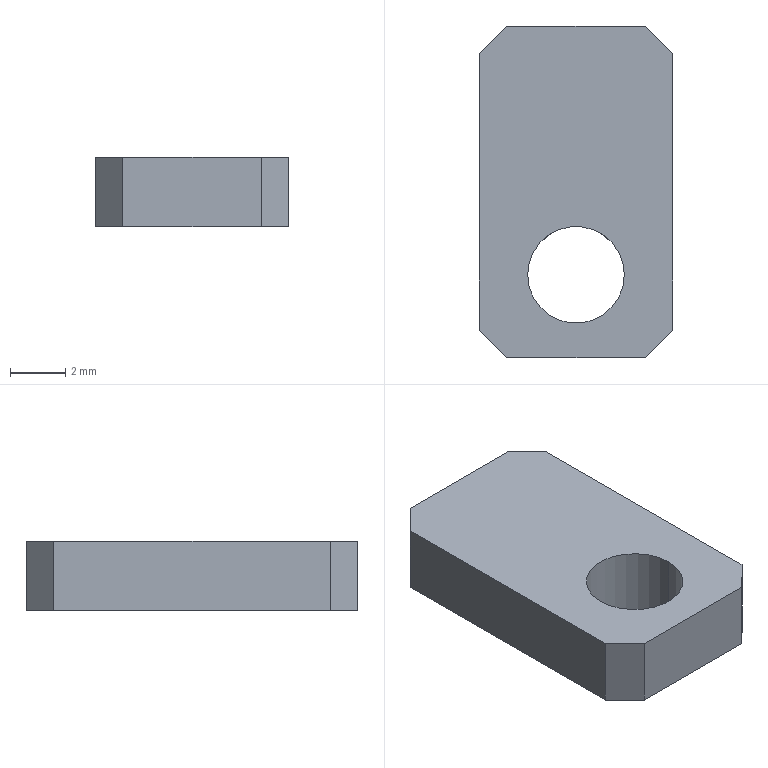Part | SolidWorks | features Chamfer 1, Extrusion 1, HoleWzd 1 | 1 solid | 12 faces | box 7 x 12 x 2.5 mm | volume 180.947 mm3 | plane 10 | cylinder 2 | commonest cylinder face diameters 3.5 x2
STEP:
#1=CARTESIAN_POINT('',(-1.75,-3.,-1.25));
#2=VERTEX_POINT('',#1);
#3=CARTESIAN_POINT('',(1.75,-3.,-1.25));
#4=VERTEX_POINT('',#3);
#5=CARTESIAN_POINT('',(0.,-3.,-1.25));
#6=DIRECTION('',(0.,0.,1.));
#7=DIRECTION('',(1.,0.,0.));
#8=AXIS2_PLACEMENT_3D('',#5,#6,#7);
#9=CIRCLE('',#8,1.75);
#10=EDGE_CURVE('',#2,#4,#9,.T.);
#11=ORIENTED_EDGE('',*,*,#10,.F.);
#12=CARTESIAN_POINT('',(-1.75,-3.,1.25));
#13=VERTEX_POINT('',#12);
#14=CARTESIAN_POINT('',(-1.75,-3.,1.25));
#15=DIRECTION('',(0.,0.,1.));
#16=VECTOR('',#15,1000.);
#17=LINE('',#14,#16);
#18=EDGE_CURVE('',#2,#13,#17,.T.);
#19=ORIENTED_EDGE('',*,*,#18,.T.);
#20=CARTESIAN_POINT('',(1.75,-3.,1.25));
#21=VERTEX_POINT('',#20);
#22=CARTESIAN_POINT('',(0.,-3.,1.25));
#23=DIRECTION('',(0.,0.,1.));
#24=DIRECTION('',(1.,0.,0.));
#25=AXIS2_PLACEMENT_3D('',#22,#23,#24);
#26=CIRCLE('',#25,1.75);
#27=EDGE_CURVE('',#13,#21,#26,.T.);
#28=ORIENTED_EDGE('',*,*,#27,.T.);
#29=CARTESIAN_POINT('',(1.75,-3.,1.25));
#30=DIRECTION('',(0.,0.,1.));
#31=VECTOR('',#30,1000.);
#32=LINE('',#29,#31);
#33=EDGE_CURVE('',#4,#21,#32,.T.);
#34=ORIENTED_EDGE('',*,*,#33,.F.);
#35=EDGE_LOOP('',(#11,#19,#28,#34));
#36=FACE_OUTER_BOUND('',#35,.T.);
#37=CARTESIAN_POINT('',(0.,-3.,1.25));
#38=DIRECTION('',(0.,0.,1.));
#39=DIRECTION('',(1.,0.,0.));
#40=AXIS2_PLACEMENT_3D('',#37,#38,#39);
#41=CYLINDRICAL_SURFACE('',#40,1.75);
#42=ADVANCED_FACE('',(#36),#41,.F.);
#43=CARTESIAN_POINT('',(3.5,-5.,1.25));
#44=VERTEX_POINT('',#43);
#45=CARTESIAN_POINT('',(3.5,5.,1.25));
#46=VERTEX_POINT('',#45);
#47=CARTESIAN_POINT('',(3.5,6.,1.25));
#48=DIRECTION('',(0.,1.,0.));
#49=VECTOR('',#48,1000.);
#50=LINE('',#47,#49);
#51=EDGE_CURVE('',#44,#46,#50,.T.);
#52=ORIENTED_EDGE('',*,*,#51,.F.);
#53=CARTESIAN_POINT('',(3.5,-5.,-1.25));
#54=VERTEX_POINT('',#53);
#55=CARTESIAN_POINT('',(3.5,-5.,1.25));
#56=DIRECTION('',(0.,0.,-1.));
#57=VECTOR('',#56,1000.);
#58=LINE('',#55,#57);
#59=EDGE_CURVE('',#44,#54,#58,.T.);
#60=ORIENTED_EDGE('',*,*,#59,.T.);
#61=CARTESIAN_POINT('',(3.5,5.,-1.25));
#62=VERTEX_POINT('',#61);
#63=CARTESIAN_POINT('',(3.5,6.,-1.25));
#64=DIRECTION('',(0.,1.,0.));
#65=VECTOR('',#64,1000.);
#66=LINE('',#63,#65);
#67=EDGE_CURVE('',#54,#62,#66,.T.);
#68=ORIENTED_EDGE('',*,*,#67,.T.);
#69=CARTESIAN_POINT('',(3.5,5.,1.25));
#70=DIRECTION('',(0.,0.,1.));
#71=VECTOR('',#70,1000.);
#72=LINE('',#69,#71);
#73=EDGE_CURVE('',#62,#46,#72,.T.);
#74=ORIENTED_EDGE('',*,*,#73,.T.);
#75=EDGE_LOOP('',(#52,#60,#68,#74));
#76=FACE_OUTER_BOUND('',#75,.T.);
#77=CARTESIAN_POINT('',(3.5,6.,1.25));
#78=DIRECTION('',(-1.,0.,0.));
#79=DIRECTION('',(0.,-1.,0.));
#80=AXIS2_PLACEMENT_3D('',#77,#78,#79);
#81=PLANE('',#80);
#82=ADVANCED_FACE('',(#76),#81,.F.);
#83=CARTESIAN_POINT('',(2.5,6.,-1.25));
#84=VERTEX_POINT('',#83);
#85=CARTESIAN_POINT('',(-2.5,6.,-1.25));
#86=VERTEX_POINT('',#85);
#87=CARTESIAN_POINT('',(-3.5,6.,-1.25));
#88=DIRECTION('',(-1.,0.,0.));
#89=VECTOR('',#88,1000.);
#90=LINE('',#87,#89);
#91=EDGE_CURVE('',#84,#86,#90,.T.);
#92=ORIENTED_EDGE('',*,*,#91,.T.);
#93=CARTESIAN_POINT('',(-2.5,6.,1.25));
#94=VERTEX_POINT('',#93);
#95=CARTESIAN_POINT('',(-2.5,6.,1.25));
#96=DIRECTION('',(0.,0.,1.));
#97=VECTOR('',#96,1000.);
#98=LINE('',#95,#97);
#99=EDGE_CURVE('',#86,#94,#98,.T.);
#100=ORIENTED_EDGE('',*,*,#99,.T.);
#101=CARTESIAN_POINT('',(2.5,6.,1.25));
#102=VERTEX_POINT('',#101);
#103=CARTESIAN_POINT('',(-3.5,6.,1.25));
#104=DIRECTION('',(-1.,0.,0.));
#105=VECTOR('',#104,1000.);
#106=LINE('',#103,#105);
#107=EDGE_CURVE('',#102,#94,#106,.T.);
#108=ORIENTED_EDGE('',*,*,#107,.F.);
#109=CARTESIAN_POINT('',(2.5,6.,1.25));
#110=DIRECTION('',(0.,0.,-1.));
#111=VECTOR('',#110,1000.);
#112=LINE('',#109,#111);
#113=EDGE_CURVE('',#102,#84,#112,.T.);
#114=ORIENTED_EDGE('',*,*,#113,.T.);
#115=EDGE_LOOP('',(#92,#100,#108,#114));
#116=FACE_OUTER_BOUND('',#115,.T.);
#117=CARTESIAN_POINT('',(-3.5,6.,1.25));
#118=DIRECTION('',(0.,-1.,0.));
#119=DIRECTION('',(0.,0.,-1.));
#120=AXIS2_PLACEMENT_3D('',#117,#118,#119);
#121=PLANE('',#120);
#122=ADVANCED_FACE('',(#116),#121,.F.);
#123=CARTESIAN_POINT('',(-3.5,5.,-1.25));
#124=VERTEX_POINT('',#123);
#125=CARTESIAN_POINT('',(-3.5,-5.,-1.25));
#126=VERTEX_POINT('',#125);
#127=CARTESIAN_POINT('',(-3.5,6.,-1.25));
#128=DIRECTION('',(0.,-1.,0.));
#129=VECTOR('',#128,1000.);
#130=LINE('',#127,#129);
#131=EDGE_CURVE('',#124,#126,#130,.T.);
#132=ORIENTED_EDGE('',*,*,#131,.T.);
#133=CARTESIAN_POINT('',(-3.5,-5.,1.25));
#134=VERTEX_POINT('',#133);
#135=CARTESIAN_POINT('',(-3.5,-5.,1.25));
#136=DIRECTION('',(0.,0.,1.));
#137=VECTOR('',#136,1000.);
#138=LINE('',#135,#137);
#139=EDGE_CURVE('',#126,#134,#138,.T.);
#140=ORIENTED_EDGE('',*,*,#139,.T.);
#141=CARTESIAN_POINT('',(-3.5,5.,1.25));
#142=VERTEX_POINT('',#141);
#143=CARTESIAN_POINT('',(-3.5,6.,1.25));
#144=DIRECTION('',(0.,-1.,0.));
#145=VECTOR('',#144,1000.);
#146=LINE('',#143,#145);
#147=EDGE_CURVE('',#142,#134,#146,.T.);
#148=ORIENTED_EDGE('',*,*,#147,.F.);
#149=CARTESIAN_POINT('',(-3.5,5.,1.25));
#150=DIRECTION('',(0.,0.,-1.));
#151=VECTOR('',#150,1000.);
#152=LINE('',#149,#151);
#153=EDGE_CURVE('',#142,#124,#152,.T.);
#154=ORIENTED_EDGE('',*,*,#153,.T.);
#155=EDGE_LOOP('',(#132,#140,#148,#154));
#156=FACE_OUTER_BOUND('',#155,.T.);
#157=CARTESIAN_POINT('',(-3.5,6.,1.25));
#158=DIRECTION('',(1.,0.,0.));
#159=DIRECTION('',(0.,1.,0.));
#160=AXIS2_PLACEMENT_3D('',#157,#158,#159);
#161=PLANE('',#160);
#162=ADVANCED_FACE('',(#156),#161,.F.);
#163=CARTESIAN_POINT('',(-2.5,-6.,1.25));
#164=VERTEX_POINT('',#163);
#165=CARTESIAN_POINT('',(2.5,-6.,1.25));
#166=VERTEX_POINT('',#165);
#167=CARTESIAN_POINT('',(-3.5,-6.,1.25));
#168=DIRECTION('',(1.,0.,0.));
#169=VECTOR('',#168,1000.);
#170=LINE('',#167,#169);
#171=EDGE_CURVE('',#164,#166,#170,.T.);
#172=ORIENTED_EDGE('',*,*,#171,.F.);
#173=CARTESIAN_POINT('',(-2.5,-6.,-1.25));
#174=VERTEX_POINT('',#173);
#175=CARTESIAN_POINT('',(-2.5,-6.,1.25));
#176=DIRECTION('',(0.,0.,-1.));
#177=VECTOR('',#176,1000.);
#178=LINE('',#175,#177);
#179=EDGE_CURVE('',#164,#174,#178,.T.);
#180=ORIENTED_EDGE('',*,*,#179,.T.);
#181=CARTESIAN_POINT('',(2.5,-6.,-1.25));
#182=VERTEX_POINT('',#181);
#183=CARTESIAN_POINT('',(-3.5,-6.,-1.25));
#184=DIRECTION('',(1.,0.,0.));
#185=VECTOR('',#184,1000.);
#186=LINE('',#183,#185);
#187=EDGE_CURVE('',#174,#182,#186,.T.);
#188=ORIENTED_EDGE('',*,*,#187,.T.);
#189=CARTESIAN_POINT('',(2.5,-6.,1.25));
#190=DIRECTION('',(0.,0.,1.));
#191=VECTOR('',#190,1000.);
#192=LINE('',#189,#191);
#193=EDGE_CURVE('',#182,#166,#192,.T.);
#194=ORIENTED_EDGE('',*,*,#193,.T.);
#195=EDGE_LOOP('',(#172,#180,#188,#194));
#196=FACE_OUTER_BOUND('',#195,.T.);
#197=CARTESIAN_POINT('',(-3.5,-6.,1.25));
#198=DIRECTION('',(0.,1.,0.));
#199=DIRECTION('',(0.,0.,1.));
#200=AXIS2_PLACEMENT_3D('',#197,#198,#199);
#201=PLANE('',#200);
#202=ADVANCED_FACE('',(#196),#201,.F.);
#203=CARTESIAN_POINT('',(0.,-3.,1.25));
#204=DIRECTION('',(0.,0.,1.));
#205=DIRECTION('',(1.,0.,0.));
#206=AXIS2_PLACEMENT_3D('',#203,#204,#205);
#207=CIRCLE('',#206,1.75);
#208=EDGE_CURVE('',#21,#13,#207,.T.);
#209=ORIENTED_EDGE('',*,*,#208,.F.);
#210=ORIENTED_EDGE('',*,*,#27,.F.);
#211=EDGE_LOOP('',(#209,#210));
#212=FACE_BOUND('',#211,.T.);
#213=ORIENTED_EDGE('',*,*,#147,.T.);
#214=CARTESIAN_POINT('',(-4.25,-4.25,1.25));
#215=DIRECTION('',(0.7071,-0.7071,0.));
#216=VECTOR('',#215,1000.);
#217=LINE('',#214,#216);
#218=EDGE_CURVE('',#134,#164,#217,.T.);
#219=ORIENTED_EDGE('',*,*,#218,.T.);
#220=ORIENTED_EDGE('',*,*,#171,.T.);
#221=CARTESIAN_POINT('',(4.25,-4.25,1.25));
#222=DIRECTION('',(0.7071,0.7071,0.));
#223=VECTOR('',#222,1000.);
#224=LINE('',#221,#223);
#225=EDGE_CURVE('',#166,#44,#224,.T.);
#226=ORIENTED_EDGE('',*,*,#225,.T.);
#227=ORIENTED_EDGE('',*,*,#51,.T.);
#228=CARTESIAN_POINT('',(4.25,4.25,1.25));
#229=DIRECTION('',(-0.7071,0.7071,0.));
#230=VECTOR('',#229,1000.);
#231=LINE('',#228,#230);
#232=EDGE_CURVE('',#46,#102,#231,.T.);
#233=ORIENTED_EDGE('',*,*,#232,.T.);
#234=ORIENTED_EDGE('',*,*,#107,.T.);
#235=CARTESIAN_POINT('',(-4.25,4.25,1.25));
#236=DIRECTION('',(-0.7071,-0.7071,0.));
#237=VECTOR('',#236,1000.);
#238=LINE('',#235,#237);
#239=EDGE_CURVE('',#94,#142,#238,.T.);
#240=ORIENTED_EDGE('',*,*,#239,.T.);
#241=EDGE_LOOP('',(#213,#219,#220,#226,#227,#233,#234,#240));
#242=FACE_OUTER_BOUND('',#241,.T.);
#243=CARTESIAN_POINT('',(0.,0.,1.25));
#244=DIRECTION('',(0.,0.,1.));
#245=DIRECTION('',(1.,0.,0.));
#246=AXIS2_PLACEMENT_3D('',#243,#244,#245);
#247=PLANE('',#246);
#248=ADVANCED_FACE('',(#212,#242),#247,.T.);
#249=CARTESIAN_POINT('',(0.,-3.,-1.25));
#250=DIRECTION('',(0.,0.,1.));
#251=DIRECTION('',(1.,0.,0.));
#252=AXIS2_PLACEMENT_3D('',#249,#250,#251);
#253=CIRCLE('',#252,1.75);
#254=EDGE_CURVE('',#4,#2,#253,.T.);
#255=ORIENTED_EDGE('',*,*,#254,.T.);
#256=ORIENTED_EDGE('',*,*,#10,.T.);
#257=EDGE_LOOP('',(#255,#256));
#258=FACE_BOUND('',#257,.T.);
#259=ORIENTED_EDGE('',*,*,#187,.F.);
#260=CARTESIAN_POINT('',(-2.5,-6.,-1.25));
#261=DIRECTION('',(-0.7071,0.7071,0.));
#262=VECTOR('',#261,1000.);
#263=LINE('',#260,#262);
#264=EDGE_CURVE('',#174,#126,#263,.T.);
#265=ORIENTED_EDGE('',*,*,#264,.T.);
#266=ORIENTED_EDGE('',*,*,#131,.F.);
#267=CARTESIAN_POINT('',(-3.5,5.,-1.25));
#268=DIRECTION('',(0.7071,0.7071,0.));
#269=VECTOR('',#268,1000.);
#270=LINE('',#267,#269);
#271=EDGE_CURVE('',#124,#86,#270,.T.);
#272=ORIENTED_EDGE('',*,*,#271,.T.);
#273=ORIENTED_EDGE('',*,*,#91,.F.);
#274=CARTESIAN_POINT('',(2.5,6.,-1.25));
#275=DIRECTION('',(0.7071,-0.7071,0.));
#276=VECTOR('',#275,1000.);
#277=LINE('',#274,#276);
#278=EDGE_CURVE('',#84,#62,#277,.T.);
#279=ORIENTED_EDGE('',*,*,#278,.T.);
#280=ORIENTED_EDGE('',*,*,#67,.F.);
#281=CARTESIAN_POINT('',(3.5,-5.,-1.25));
#282=DIRECTION('',(-0.7071,-0.7071,0.));
#283=VECTOR('',#282,1000.);
#284=LINE('',#281,#283);
#285=EDGE_CURVE('',#54,#182,#284,.T.);
#286=ORIENTED_EDGE('',*,*,#285,.T.);
#287=EDGE_LOOP('',(#259,#265,#266,#272,#273,#279,#280,#286));
#288=FACE_OUTER_BOUND('',#287,.T.);
#289=CARTESIAN_POINT('',(0.,0.,-1.25));
#290=DIRECTION('',(0.,0.,1.));
#291=DIRECTION('',(1.,0.,0.));
#292=AXIS2_PLACEMENT_3D('',#289,#290,#291);
#293=PLANE('',#292);
#294=ADVANCED_FACE('',(#258,#288),#293,.F.);
#295=ORIENTED_EDGE('',*,*,#18,.F.);
#296=ORIENTED_EDGE('',*,*,#254,.F.);
#297=ORIENTED_EDGE('',*,*,#33,.T.);
#298=ORIENTED_EDGE('',*,*,#208,.T.);
#299=EDGE_LOOP('',(#295,#296,#297,#298));
#300=FACE_OUTER_BOUND('',#299,.T.);
#301=CARTESIAN_POINT('',(0.,-3.,1.25));
#302=DIRECTION('',(0.,0.,1.));
#303=DIRECTION('',(1.,0.,0.));
#304=AXIS2_PLACEMENT_3D('',#301,#302,#303);
#305=CYLINDRICAL_SURFACE('',#304,1.75);
#306=ADVANCED_FACE('',(#300),#305,.F.);
#307=ORIENTED_EDGE('',*,*,#218,.F.);
#308=ORIENTED_EDGE('',*,*,#139,.F.);
#309=ORIENTED_EDGE('',*,*,#264,.F.);
#310=ORIENTED_EDGE('',*,*,#179,.F.);
#311=EDGE_LOOP('',(#307,#308,#309,#310));
#312=FACE_OUTER_BOUND('',#311,.T.);
#313=CARTESIAN_POINT('',(-2.5,-6.,1.25));
#314=DIRECTION('',(0.7071,0.7071,0.));
#315=DIRECTION('',(0.,0.,-1.));
#316=AXIS2_PLACEMENT_3D('',#313,#314,#315);
#317=PLANE('',#316);
#318=ADVANCED_FACE('',(#312),#317,.F.);
#319=ORIENTED_EDGE('',*,*,#225,.F.);
#320=ORIENTED_EDGE('',*,*,#193,.F.);
#321=ORIENTED_EDGE('',*,*,#285,.F.);
#322=ORIENTED_EDGE('',*,*,#59,.F.);
#323=EDGE_LOOP('',(#319,#320,#321,#322));
#324=FACE_OUTER_BOUND('',#323,.T.);
#325=CARTESIAN_POINT('',(3.5,-5.,1.25));
#326=DIRECTION('',(-0.7071,0.7071,0.));
#327=DIRECTION('',(0.,0.,-1.));
#328=AXIS2_PLACEMENT_3D('',#325,#326,#327);
#329=PLANE('',#328);
#330=ADVANCED_FACE('',(#324),#329,.F.);
#331=ORIENTED_EDGE('',*,*,#239,.F.);
#332=ORIENTED_EDGE('',*,*,#99,.F.);
#333=ORIENTED_EDGE('',*,*,#271,.F.);
#334=ORIENTED_EDGE('',*,*,#153,.F.);
#335=EDGE_LOOP('',(#331,#332,#333,#334));
#336=FACE_OUTER_BOUND('',#335,.T.);
#337=CARTESIAN_POINT('',(-3.5,5.,1.25));
#338=DIRECTION('',(0.7071,-0.7071,0.));
#339=DIRECTION('',(0.,0.,-1.));
#340=AXIS2_PLACEMENT_3D('',#337,#338,#339);
#341=PLANE('',#340);
#342=ADVANCED_FACE('',(#336),#341,.F.);
#343=ORIENTED_EDGE('',*,*,#232,.F.);
#344=ORIENTED_EDGE('',*,*,#73,.F.);
#345=ORIENTED_EDGE('',*,*,#278,.F.);
#346=ORIENTED_EDGE('',*,*,#113,.F.);
#347=EDGE_LOOP('',(#343,#344,#345,#346));
#348=FACE_OUTER_BOUND('',#347,.T.);
#349=CARTESIAN_POINT('',(2.5,6.,1.25));
#350=DIRECTION('',(-0.7071,-0.7071,0.));
#351=DIRECTION('',(0.,0.,-1.));
#352=AXIS2_PLACEMENT_3D('',#349,#350,#351);
#353=PLANE('',#352);
#354=ADVANCED_FACE('',(#348),#353,.F.);
#355=CLOSED_SHELL('',(#42,#82,#122,#162,#202,#248,#294,#306,#318,#330,#342,#354));
#356=MANIFOLD_SOLID_BREP('',#355);
#357=CARTESIAN_POINT('',(0.,0.,0.));
#358=DIRECTION('',(0.,0.,1.));
#359=DIRECTION('',(1.,0.,0.));
#360=AXIS2_PLACEMENT_3D('',#357,#358,#359);
#361=(LENGTH_UNIT()NAMED_UNIT(*)SI_UNIT(.MILLI.,.METRE.));
#362=UNCERTAINTY_MEASURE_WITH_UNIT(LENGTH_MEASURE(0.00001),#361,'','');
#363=(NAMED_UNIT(*)PLANE_ANGLE_UNIT()SI_UNIT($,.RADIAN.));
#364=(NAMED_UNIT(*)SI_UNIT($,.STERADIAN.)SOLID_ANGLE_UNIT());
#365=(GEOMETRIC_REPRESENTATION_CONTEXT(3)GLOBAL_UNCERTAINTY_ASSIGNED_CONTEXT((#362))GLOBAL_UNIT_ASSIGNED_CONTEXT((#361,#363,#364))REPRESENTATION_CONTEXT('',''));
#366=ADVANCED_BREP_SHAPE_REPRESENTATION('',(#356,#360),#365);